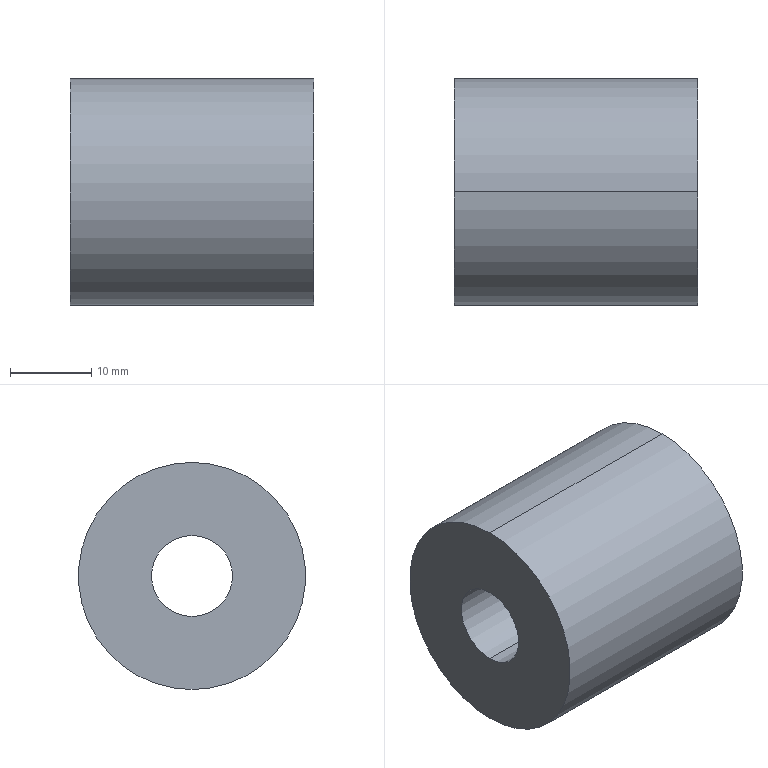Part | SolidWorks | features BaseBody 1 | 1 solid | 6 faces | box 30 x 28 x 28 mm | volume 16116 mm3 | cylinder 4 | plane 2 | commonest cylinder face diameters 10 x2 28 x2
STEP:
#1=CARTESIAN_POINT('',(104.,-12.,43.));
#2=VERTEX_POINT('',#1);
#3=CARTESIAN_POINT('',(104.,-12.,71.));
#4=VERTEX_POINT('',#3);
#5=CARTESIAN_POINT('',(104.,-12.,57.));
#6=DIRECTION('',(1.,0.,0.));
#7=DIRECTION('',(0.,0.,-1.));
#8=AXIS2_PLACEMENT_3D('',#5,#6,#7);
#9=CIRCLE('',#8,14.);
#10=EDGE_CURVE('',#2,#4,#9,.T.);
#11=ORIENTED_EDGE('',*,*,#10,.T.);
#12=CARTESIAN_POINT('',(134.,-12.,71.));
#13=VERTEX_POINT('',#12);
#14=CARTESIAN_POINT('',(104.,-12.,71.));
#15=DIRECTION('',(1.,0.,0.));
#16=VECTOR('',#15,1000.);
#17=LINE('',#14,#16);
#18=EDGE_CURVE('',#4,#13,#17,.T.);
#19=ORIENTED_EDGE('',*,*,#18,.T.);
#20=CARTESIAN_POINT('',(134.,-12.,43.));
#21=VERTEX_POINT('',#20);
#22=CARTESIAN_POINT('',(134.,-12.,57.));
#23=DIRECTION('',(-1.,0.,0.));
#24=DIRECTION('',(0.,0.,-1.));
#25=AXIS2_PLACEMENT_3D('',#22,#23,#24);
#26=CIRCLE('',#25,14.);
#27=EDGE_CURVE('',#13,#21,#26,.T.);
#28=ORIENTED_EDGE('',*,*,#27,.T.);
#29=CARTESIAN_POINT('',(104.,-12.,43.));
#30=DIRECTION('',(1.,0.,0.));
#31=VECTOR('',#30,1000.);
#32=LINE('',#29,#31);
#33=EDGE_CURVE('',#2,#21,#32,.T.);
#34=ORIENTED_EDGE('',*,*,#33,.F.);
#35=EDGE_LOOP('',(#11,#19,#28,#34));
#36=FACE_OUTER_BOUND('',#35,.T.);
#37=CARTESIAN_POINT('',(104.,-12.,57.));
#38=DIRECTION('',(1.,0.,0.));
#39=DIRECTION('',(0.,0.,-1.));
#40=AXIS2_PLACEMENT_3D('',#37,#38,#39);
#41=CYLINDRICAL_SURFACE('',#40,14.);
#42=ADVANCED_FACE('',(#36),#41,.T.);
#43=CARTESIAN_POINT('',(104.,-12.,52.));
#44=VERTEX_POINT('',#43);
#45=CARTESIAN_POINT('',(104.,-12.,62.));
#46=VERTEX_POINT('',#45);
#47=CARTESIAN_POINT('',(104.,-12.,57.));
#48=DIRECTION('',(-1.,0.,0.));
#49=DIRECTION('',(0.,0.,-1.));
#50=AXIS2_PLACEMENT_3D('',#47,#48,#49);
#51=CIRCLE('',#50,5.);
#52=EDGE_CURVE('',#44,#46,#51,.T.);
#53=ORIENTED_EDGE('',*,*,#52,.T.);
#54=CARTESIAN_POINT('',(134.,-12.,62.));
#55=VERTEX_POINT('',#54);
#56=CARTESIAN_POINT('',(104.,-12.,62.));
#57=DIRECTION('',(1.,0.,0.));
#58=VECTOR('',#57,1000.);
#59=LINE('',#56,#58);
#60=EDGE_CURVE('',#46,#55,#59,.T.);
#61=ORIENTED_EDGE('',*,*,#60,.T.);
#62=CARTESIAN_POINT('',(134.,-12.,52.));
#63=VERTEX_POINT('',#62);
#64=CARTESIAN_POINT('',(134.,-12.,57.));
#65=DIRECTION('',(-1.,0.,0.));
#66=DIRECTION('',(0.,0.,-1.));
#67=AXIS2_PLACEMENT_3D('',#64,#65,#66);
#68=CIRCLE('',#67,5.);
#69=EDGE_CURVE('',#63,#55,#68,.T.);
#70=ORIENTED_EDGE('',*,*,#69,.F.);
#71=CARTESIAN_POINT('',(104.,-12.,52.));
#72=DIRECTION('',(1.,0.,0.));
#73=VECTOR('',#72,1000.);
#74=LINE('',#71,#73);
#75=EDGE_CURVE('',#44,#63,#74,.T.);
#76=ORIENTED_EDGE('',*,*,#75,.F.);
#77=EDGE_LOOP('',(#53,#61,#70,#76));
#78=FACE_OUTER_BOUND('',#77,.T.);
#79=CARTESIAN_POINT('',(104.,-12.,57.));
#80=DIRECTION('',(1.,0.,0.));
#81=DIRECTION('',(0.,0.,-1.));
#82=AXIS2_PLACEMENT_3D('',#79,#80,#81);
#83=CYLINDRICAL_SURFACE('',#82,5.);
#84=ADVANCED_FACE('',(#78),#83,.F.);
#85=ORIENTED_EDGE('',*,*,#18,.F.);
#86=CARTESIAN_POINT('',(104.,-12.,57.));
#87=DIRECTION('',(1.,0.,0.));
#88=DIRECTION('',(0.,0.,-1.));
#89=AXIS2_PLACEMENT_3D('',#86,#87,#88);
#90=CIRCLE('',#89,14.);
#91=EDGE_CURVE('',#4,#2,#90,.T.);
#92=ORIENTED_EDGE('',*,*,#91,.T.);
#93=ORIENTED_EDGE('',*,*,#33,.T.);
#94=CARTESIAN_POINT('',(134.,-12.,57.));
#95=DIRECTION('',(-1.,0.,0.));
#96=DIRECTION('',(0.,0.,-1.));
#97=AXIS2_PLACEMENT_3D('',#94,#95,#96);
#98=CIRCLE('',#97,14.);
#99=EDGE_CURVE('',#21,#13,#98,.T.);
#100=ORIENTED_EDGE('',*,*,#99,.T.);
#101=EDGE_LOOP('',(#85,#92,#93,#100));
#102=FACE_OUTER_BOUND('',#101,.T.);
#103=CARTESIAN_POINT('',(104.,-12.,57.));
#104=DIRECTION('',(1.,0.,0.));
#105=DIRECTION('',(0.,0.,-1.));
#106=AXIS2_PLACEMENT_3D('',#103,#104,#105);
#107=CYLINDRICAL_SURFACE('',#106,14.);
#108=ADVANCED_FACE('',(#102),#107,.T.);
#109=ORIENTED_EDGE('',*,*,#52,.F.);
#110=CARTESIAN_POINT('',(104.,-12.,57.));
#111=DIRECTION('',(-1.,0.,0.));
#112=DIRECTION('',(0.,0.,-1.));
#113=AXIS2_PLACEMENT_3D('',#110,#111,#112);
#114=CIRCLE('',#113,5.);
#115=EDGE_CURVE('',#46,#44,#114,.T.);
#116=ORIENTED_EDGE('',*,*,#115,.F.);
#117=EDGE_LOOP('',(#109,#116));
#118=FACE_BOUND('',#117,.T.);
#119=ORIENTED_EDGE('',*,*,#10,.F.);
#120=ORIENTED_EDGE('',*,*,#91,.F.);
#121=EDGE_LOOP('',(#119,#120));
#122=FACE_OUTER_BOUND('',#121,.T.);
#123=CARTESIAN_POINT('',(104.,-12.,57.));
#124=DIRECTION('',(1.,0.,0.));
#125=DIRECTION('',(0.,0.,-1.));
#126=AXIS2_PLACEMENT_3D('',#123,#124,#125);
#127=PLANE('',#126);
#128=ADVANCED_FACE('',(#118,#122),#127,.F.);
#129=ORIENTED_EDGE('',*,*,#69,.T.);
#130=CARTESIAN_POINT('',(134.,-12.,57.));
#131=DIRECTION('',(-1.,0.,0.));
#132=DIRECTION('',(0.,0.,-1.));
#133=AXIS2_PLACEMENT_3D('',#130,#131,#132);
#134=CIRCLE('',#133,5.);
#135=EDGE_CURVE('',#55,#63,#134,.T.);
#136=ORIENTED_EDGE('',*,*,#135,.T.);
#137=EDGE_LOOP('',(#129,#136));
#138=FACE_BOUND('',#137,.T.);
#139=ORIENTED_EDGE('',*,*,#99,.F.);
#140=ORIENTED_EDGE('',*,*,#27,.F.);
#141=EDGE_LOOP('',(#139,#140));
#142=FACE_OUTER_BOUND('',#141,.T.);
#143=CARTESIAN_POINT('',(134.,-12.,57.));
#144=DIRECTION('',(1.,0.,0.));
#145=DIRECTION('',(0.,0.,-1.));
#146=AXIS2_PLACEMENT_3D('',#143,#144,#145);
#147=PLANE('',#146);
#148=ADVANCED_FACE('',(#138,#142),#147,.T.);
#149=ORIENTED_EDGE('',*,*,#60,.F.);
#150=ORIENTED_EDGE('',*,*,#115,.T.);
#151=ORIENTED_EDGE('',*,*,#75,.T.);
#152=ORIENTED_EDGE('',*,*,#135,.F.);
#153=EDGE_LOOP('',(#149,#150,#151,#152));
#154=FACE_OUTER_BOUND('',#153,.T.);
#155=CARTESIAN_POINT('',(104.,-12.,57.));
#156=DIRECTION('',(1.,0.,0.));
#157=DIRECTION('',(0.,0.,-1.));
#158=AXIS2_PLACEMENT_3D('',#155,#156,#157);
#159=CYLINDRICAL_SURFACE('',#158,5.);
#160=ADVANCED_FACE('',(#154),#159,.F.);
#161=CLOSED_SHELL('',(#42,#84,#108,#128,#148,#160));
#162=MANIFOLD_SOLID_BREP('',#161);
#163=CARTESIAN_POINT('',(0.,0.,0.));
#164=DIRECTION('',(0.,0.,1.));
#165=DIRECTION('',(1.,0.,0.));
#166=AXIS2_PLACEMENT_3D('',#163,#164,#165);
#167=(LENGTH_UNIT()NAMED_UNIT(*)SI_UNIT(.MILLI.,.METRE.));
#168=UNCERTAINTY_MEASURE_WITH_UNIT(LENGTH_MEASURE(0.00001),#167,'','');
#169=(NAMED_UNIT(*)PLANE_ANGLE_UNIT()SI_UNIT($,.RADIAN.));
#170=(NAMED_UNIT(*)SI_UNIT($,.STERADIAN.)SOLID_ANGLE_UNIT());
#171=(GEOMETRIC_REPRESENTATION_CONTEXT(3)GLOBAL_UNCERTAINTY_ASSIGNED_CONTEXT((#168))GLOBAL_UNIT_ASSIGNED_CONTEXT((#167,#169,#170))REPRESENTATION_CONTEXT('',''));
#172=ADVANCED_BREP_SHAPE_REPRESENTATION('',(#162,#166),#171);